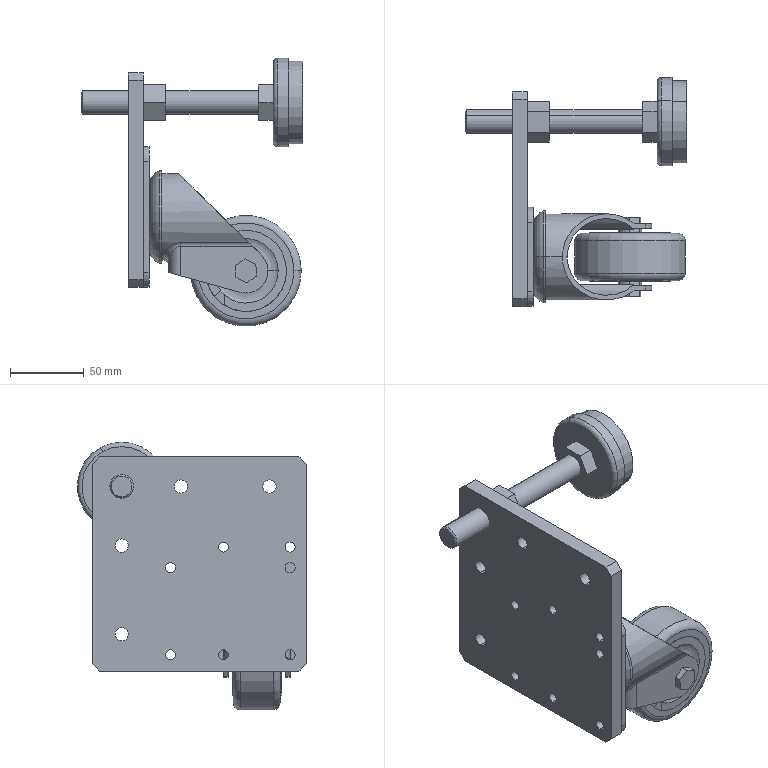Part | SolidWorks | features AEMSimFeature 1 | 6 solids | 169 faces | box 150 x 155 x 181.5 mm | volume 514877 mm3 | plane 82 | cylinder 70 | torus 13 | spline 2 | cone 2 | commonest cylinder face diameters 6.8 x14 8.636 x8 9 x8 15.875 x4 16 x4 20.32 x4